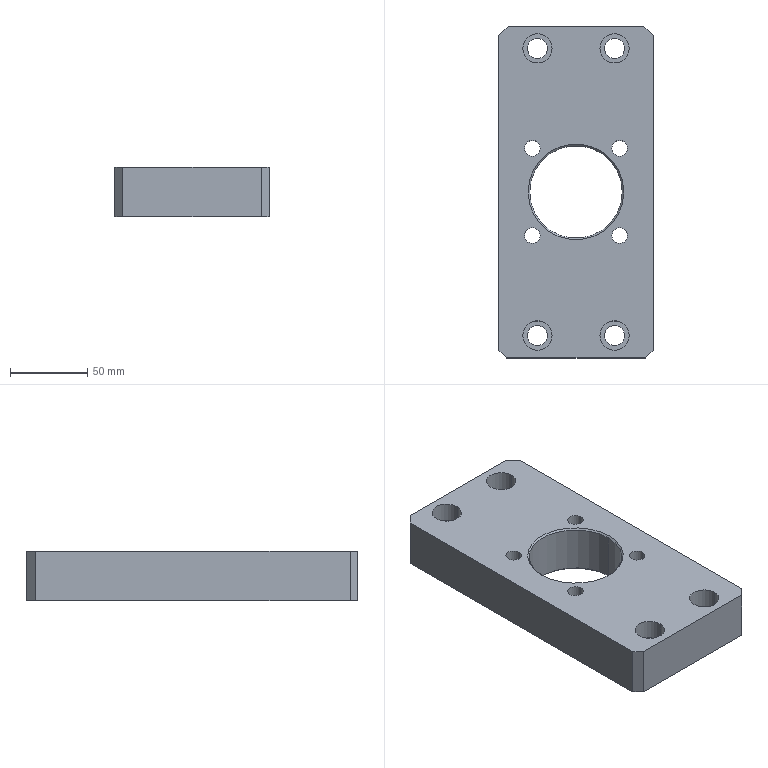Part | SolidWorks | features BaseBody 1 | 1 solid | 44 faces | box 100 x 215 x 32 mm | volume 560281 mm3 | cylinder 26 | plane 14 | cone 4 | commonest cylinder face diameters 10.106 x8 13 x8 19 x8 60 x2
STEP:
#1=CARTESIAN_POINT('',(146.031,36.728,1.));
#2=VERTEX_POINT('',#1);
#3=CARTESIAN_POINT('',(86.031,36.728,1.));
#4=VERTEX_POINT('',#3);
#5=CARTESIAN_POINT('',(116.031,36.728,1.));
#6=DIRECTION('',(0.,0.,-1.));
#7=DIRECTION('',(-1.,0.,0.));
#8=AXIS2_PLACEMENT_3D('',#5,#6,#7);
#9=CIRCLE('',#8,30.);
#10=EDGE_CURVE('',#2,#4,#9,.T.);
#11=ORIENTED_EDGE('',*,*,#10,.F.);
#12=CARTESIAN_POINT('',(147.031,36.728,0.));
#13=VERTEX_POINT('',#12);
#14=CARTESIAN_POINT('',(147.031,36.728,0.));
#15=DIRECTION('',(0.7071,0.,-0.7071));
#16=VECTOR('',#15,1000.);
#17=LINE('',#14,#16);
#18=EDGE_CURVE('',#2,#13,#17,.T.);
#19=ORIENTED_EDGE('',*,*,#18,.T.);
#20=CARTESIAN_POINT('',(85.031,36.728,0.));
#21=VERTEX_POINT('',#20);
#22=CARTESIAN_POINT('',(116.031,36.728,0.));
#23=DIRECTION('',(0.,0.,-1.));
#24=DIRECTION('',(-1.,0.,0.));
#25=AXIS2_PLACEMENT_3D('',#22,#23,#24);
#26=CIRCLE('',#25,31.);
#27=EDGE_CURVE('',#13,#21,#26,.T.);
#28=ORIENTED_EDGE('',*,*,#27,.T.);
#29=CARTESIAN_POINT('',(85.031,36.728,0.));
#30=DIRECTION('',(-0.7071,0.,-0.7071));
#31=VECTOR('',#30,1000.);
#32=LINE('',#29,#31);
#33=EDGE_CURVE('',#4,#21,#32,.T.);
#34=ORIENTED_EDGE('',*,*,#33,.F.);
#35=EDGE_LOOP('',(#11,#19,#28,#34));
#36=FACE_OUTER_BOUND('',#35,.T.);
#37=CARTESIAN_POINT('',(116.031,36.728,0.));
#38=DIRECTION('',(0.,0.,-1.));
#39=DIRECTION('',(-1.,0.,0.));
#40=AXIS2_PLACEMENT_3D('',#37,#38,#39);
#41=CONICAL_SURFACE('',#40,31.,0.7854);
#42=ADVANCED_FACE('',(#36),#41,.F.);
#43=CARTESIAN_POINT('',(92.799,8.444,0.));
#44=VERTEX_POINT('',#43);
#45=CARTESIAN_POINT('',(82.693,8.444,0.));
#46=VERTEX_POINT('',#45);
#47=CARTESIAN_POINT('',(87.746,8.444,0.));
#48=DIRECTION('',(0.,0.,-1.));
#49=DIRECTION('',(1.,0.,0.));
#50=AXIS2_PLACEMENT_3D('',#47,#48,#49);
#51=CIRCLE('',#50,5.053);
#52=EDGE_CURVE('',#44,#46,#51,.T.);
#53=ORIENTED_EDGE('',*,*,#52,.T.);
#54=CARTESIAN_POINT('',(82.693,8.444,32.));
#55=VERTEX_POINT('',#54);
#56=CARTESIAN_POINT('',(82.693,8.444,-207.268));
#57=DIRECTION('',(0.,0.,1.));
#58=VECTOR('',#57,1000.);
#59=LINE('',#56,#58);
#60=EDGE_CURVE('',#46,#55,#59,.T.);
#61=ORIENTED_EDGE('',*,*,#60,.T.);
#62=CARTESIAN_POINT('',(92.799,8.444,32.));
#63=VERTEX_POINT('',#62);
#64=CARTESIAN_POINT('',(87.746,8.444,32.));
#65=DIRECTION('',(0.,0.,-1.));
#66=DIRECTION('',(1.,0.,0.));
#67=AXIS2_PLACEMENT_3D('',#64,#65,#66);
#68=CIRCLE('',#67,5.053);
#69=EDGE_CURVE('',#63,#55,#68,.T.);
#70=ORIENTED_EDGE('',*,*,#69,.F.);
#71=CARTESIAN_POINT('',(92.799,8.444,-207.268));
#72=DIRECTION('',(0.,0.,1.));
#73=VECTOR('',#72,1000.);
#74=LINE('',#71,#73);
#75=EDGE_CURVE('',#44,#63,#74,.T.);
#76=ORIENTED_EDGE('',*,*,#75,.F.);
#77=EDGE_LOOP('',(#53,#61,#70,#76));
#78=FACE_OUTER_BOUND('',#77,.T.);
#79=CARTESIAN_POINT('',(87.746,8.444,-207.268));
#80=DIRECTION('',(0.,0.,1.));
#81=DIRECTION('',(1.,0.,0.));
#82=AXIS2_PLACEMENT_3D('',#79,#80,#81);
#83=CYLINDRICAL_SURFACE('',#82,5.053);
#84=ADVANCED_FACE('',(#78),#83,.F.);
#85=CARTESIAN_POINT('',(149.368,8.444,0.));
#86=VERTEX_POINT('',#85);
#87=CARTESIAN_POINT('',(139.262,8.444,0.));
#88=VERTEX_POINT('',#87);
#89=CARTESIAN_POINT('',(144.315,8.444,0.));
#90=DIRECTION('',(0.,0.,-1.));
#91=DIRECTION('',(1.,0.,0.));
#92=AXIS2_PLACEMENT_3D('',#89,#90,#91);
#93=CIRCLE('',#92,5.053);
#94=EDGE_CURVE('',#86,#88,#93,.T.);
#95=ORIENTED_EDGE('',*,*,#94,.T.);
#96=CARTESIAN_POINT('',(139.262,8.444,32.));
#97=VERTEX_POINT('',#96);
#98=CARTESIAN_POINT('',(139.262,8.444,-207.268));
#99=DIRECTION('',(0.,0.,1.));
#100=VECTOR('',#99,1000.);
#101=LINE('',#98,#100);
#102=EDGE_CURVE('',#88,#97,#101,.T.);
#103=ORIENTED_EDGE('',*,*,#102,.T.);
#104=CARTESIAN_POINT('',(149.368,8.444,32.));
#105=VERTEX_POINT('',#104);
#106=CARTESIAN_POINT('',(144.315,8.444,32.));
#107=DIRECTION('',(0.,0.,-1.));
#108=DIRECTION('',(1.,0.,0.));
#109=AXIS2_PLACEMENT_3D('',#106,#107,#108);
#110=CIRCLE('',#109,5.053);
#111=EDGE_CURVE('',#105,#97,#110,.T.);
#112=ORIENTED_EDGE('',*,*,#111,.F.);
#113=CARTESIAN_POINT('',(149.368,8.444,-207.268));
#114=DIRECTION('',(0.,0.,1.));
#115=VECTOR('',#114,1000.);
#116=LINE('',#113,#115);
#117=EDGE_CURVE('',#86,#105,#116,.T.);
#118=ORIENTED_EDGE('',*,*,#117,.F.);
#119=EDGE_LOOP('',(#95,#103,#112,#118));
#120=FACE_OUTER_BOUND('',#119,.T.);
#121=CARTESIAN_POINT('',(144.315,8.444,-207.268));
#122=DIRECTION('',(0.,0.,1.));
#123=DIRECTION('',(1.,0.,0.));
#124=AXIS2_PLACEMENT_3D('',#121,#122,#123);
#125=CYLINDRICAL_SURFACE('',#124,5.053);
#126=ADVANCED_FACE('',(#120),#125,.F.);
#127=CARTESIAN_POINT('',(149.368,65.013,0.));
#128=VERTEX_POINT('',#127);
#129=CARTESIAN_POINT('',(139.262,65.013,0.));
#130=VERTEX_POINT('',#129);
#131=CARTESIAN_POINT('',(144.315,65.013,0.));
#132=DIRECTION('',(0.,0.,-1.));
#133=DIRECTION('',(1.,0.,0.));
#134=AXIS2_PLACEMENT_3D('',#131,#132,#133);
#135=CIRCLE('',#134,5.053);
#136=EDGE_CURVE('',#128,#130,#135,.T.);
#137=ORIENTED_EDGE('',*,*,#136,.T.);
#138=CARTESIAN_POINT('',(139.262,65.013,32.));
#139=VERTEX_POINT('',#138);
#140=CARTESIAN_POINT('',(139.262,65.013,-207.268));
#141=DIRECTION('',(0.,0.,1.));
#142=VECTOR('',#141,1000.);
#143=LINE('',#140,#142);
#144=EDGE_CURVE('',#130,#139,#143,.T.);
#145=ORIENTED_EDGE('',*,*,#144,.T.);
#146=CARTESIAN_POINT('',(149.368,65.013,32.));
#147=VERTEX_POINT('',#146);
#148=CARTESIAN_POINT('',(144.315,65.013,32.));
#149=DIRECTION('',(0.,0.,-1.));
#150=DIRECTION('',(1.,0.,0.));
#151=AXIS2_PLACEMENT_3D('',#148,#149,#150);
#152=CIRCLE('',#151,5.053);
#153=EDGE_CURVE('',#147,#139,#152,.T.);
#154=ORIENTED_EDGE('',*,*,#153,.F.);
#155=CARTESIAN_POINT('',(149.368,65.013,-207.268));
#156=DIRECTION('',(0.,0.,1.));
#157=VECTOR('',#156,1000.);
#158=LINE('',#155,#157);
#159=EDGE_CURVE('',#128,#147,#158,.T.);
#160=ORIENTED_EDGE('',*,*,#159,.F.);
#161=EDGE_LOOP('',(#137,#145,#154,#160));
#162=FACE_OUTER_BOUND('',#161,.T.);
#163=CARTESIAN_POINT('',(144.315,65.013,-207.268));
#164=DIRECTION('',(0.,0.,1.));
#165=DIRECTION('',(1.,0.,0.));
#166=AXIS2_PLACEMENT_3D('',#163,#164,#165);
#167=CYLINDRICAL_SURFACE('',#166,5.053);
#168=ADVANCED_FACE('',(#162),#167,.F.);
#169=CARTESIAN_POINT('',(92.799,65.013,0.));
#170=VERTEX_POINT('',#169);
#171=CARTESIAN_POINT('',(82.693,65.013,0.));
#172=VERTEX_POINT('',#171);
#173=CARTESIAN_POINT('',(87.746,65.013,0.));
#174=DIRECTION('',(0.,0.,-1.));
#175=DIRECTION('',(1.,0.,0.));
#176=AXIS2_PLACEMENT_3D('',#173,#174,#175);
#177=CIRCLE('',#176,5.053);
#178=EDGE_CURVE('',#170,#172,#177,.T.);
#179=ORIENTED_EDGE('',*,*,#178,.T.);
#180=CARTESIAN_POINT('',(82.693,65.013,32.));
#181=VERTEX_POINT('',#180);
#182=CARTESIAN_POINT('',(82.693,65.013,-207.268));
#183=DIRECTION('',(0.,0.,1.));
#184=VECTOR('',#183,1000.);
#185=LINE('',#182,#184);
#186=EDGE_CURVE('',#172,#181,#185,.T.);
#187=ORIENTED_EDGE('',*,*,#186,.T.);
#188=CARTESIAN_POINT('',(92.799,65.013,32.));
#189=VERTEX_POINT('',#188);
#190=CARTESIAN_POINT('',(87.746,65.013,32.));
#191=DIRECTION('',(0.,0.,-1.));
#192=DIRECTION('',(1.,0.,0.));
#193=AXIS2_PLACEMENT_3D('',#190,#191,#192);
#194=CIRCLE('',#193,5.053);
#195=EDGE_CURVE('',#189,#181,#194,.T.);
#196=ORIENTED_EDGE('',*,*,#195,.F.);
#197=CARTESIAN_POINT('',(92.799,65.013,-207.268));
#198=DIRECTION('',(0.,0.,1.));
#199=VECTOR('',#198,1000.);
#200=LINE('',#197,#199);
#201=EDGE_CURVE('',#170,#189,#200,.T.);
#202=ORIENTED_EDGE('',*,*,#201,.F.);
#203=EDGE_LOOP('',(#179,#187,#196,#202));
#204=FACE_OUTER_BOUND('',#203,.T.);
#205=CARTESIAN_POINT('',(87.746,65.013,-207.268));
#206=DIRECTION('',(0.,0.,1.));
#207=DIRECTION('',(1.,0.,0.));
#208=AXIS2_PLACEMENT_3D('',#205,#206,#207);
#209=CYLINDRICAL_SURFACE('',#208,5.053);
#210=ADVANCED_FACE('',(#204),#209,.F.);
#211=CARTESIAN_POINT('',(97.531,-56.272,0.));
#212=VERTEX_POINT('',#211);
#213=CARTESIAN_POINT('',(84.531,-56.272,0.));
#214=VERTEX_POINT('',#213);
#215=CARTESIAN_POINT('',(91.031,-56.272,0.));
#216=DIRECTION('',(0.,0.,-1.));
#217=DIRECTION('',(1.,0.,0.));
#218=AXIS2_PLACEMENT_3D('',#215,#216,#217);
#219=CIRCLE('',#218,6.5);
#220=EDGE_CURVE('',#212,#214,#219,.T.);
#221=ORIENTED_EDGE('',*,*,#220,.T.);
#222=CARTESIAN_POINT('',(84.531,-56.272,19.));
#223=VERTEX_POINT('',#222);
#224=CARTESIAN_POINT('',(84.531,-56.272,-207.268));
#225=DIRECTION('',(0.,0.,1.));
#226=VECTOR('',#225,1000.);
#227=LINE('',#224,#226);
#228=EDGE_CURVE('',#214,#223,#227,.T.);
#229=ORIENTED_EDGE('',*,*,#228,.T.);
#230=CARTESIAN_POINT('',(97.531,-56.272,19.));
#231=VERTEX_POINT('',#230);
#232=CARTESIAN_POINT('',(91.031,-56.272,19.));
#233=DIRECTION('',(0.,0.,-1.));
#234=DIRECTION('',(1.,0.,0.));
#235=AXIS2_PLACEMENT_3D('',#232,#233,#234);
#236=CIRCLE('',#235,6.5);
#237=EDGE_CURVE('',#231,#223,#236,.T.);
#238=ORIENTED_EDGE('',*,*,#237,.F.);
#239=CARTESIAN_POINT('',(97.531,-56.272,-207.268));
#240=DIRECTION('',(0.,0.,1.));
#241=VECTOR('',#240,1000.);
#242=LINE('',#239,#241);
#243=EDGE_CURVE('',#212,#231,#242,.T.);
#244=ORIENTED_EDGE('',*,*,#243,.F.);
#245=EDGE_LOOP('',(#221,#229,#238,#244));
#246=FACE_OUTER_BOUND('',#245,.T.);
#247=CARTESIAN_POINT('',(91.031,-56.272,-207.268));
#248=DIRECTION('',(0.,0.,1.));
#249=DIRECTION('',(1.,0.,0.));
#250=AXIS2_PLACEMENT_3D('',#247,#248,#249);
#251=CYLINDRICAL_SURFACE('',#250,6.5);
#252=ADVANCED_FACE('',(#246),#251,.F.);
#253=CARTESIAN_POINT('',(147.531,-56.272,0.));
#254=VERTEX_POINT('',#253);
#255=CARTESIAN_POINT('',(134.531,-56.272,0.));
#256=VERTEX_POINT('',#255);
#257=CARTESIAN_POINT('',(141.031,-56.272,0.));
#258=DIRECTION('',(0.,0.,-1.));
#259=DIRECTION('',(1.,0.,0.));
#260=AXIS2_PLACEMENT_3D('',#257,#258,#259);
#261=CIRCLE('',#260,6.5);
#262=EDGE_CURVE('',#254,#256,#261,.T.);
#263=ORIENTED_EDGE('',*,*,#262,.T.);
#264=CARTESIAN_POINT('',(134.531,-56.272,19.));
#265=VERTEX_POINT('',#264);
#266=CARTESIAN_POINT('',(134.531,-56.272,-207.268));
#267=DIRECTION('',(0.,0.,1.));
#268=VECTOR('',#267,1000.);
#269=LINE('',#266,#268);
#270=EDGE_CURVE('',#256,#265,#269,.T.);
#271=ORIENTED_EDGE('',*,*,#270,.T.);
#272=CARTESIAN_POINT('',(147.531,-56.272,19.));
#273=VERTEX_POINT('',#272);
#274=CARTESIAN_POINT('',(141.031,-56.272,19.));
#275=DIRECTION('',(0.,0.,-1.));
#276=DIRECTION('',(1.,0.,0.));
#277=AXIS2_PLACEMENT_3D('',#274,#275,#276);
#278=CIRCLE('',#277,6.5);
#279=EDGE_CURVE('',#273,#265,#278,.T.);
#280=ORIENTED_EDGE('',*,*,#279,.F.);
#281=CARTESIAN_POINT('',(147.531,-56.272,-207.268));
#282=DIRECTION('',(0.,0.,1.));
#283=VECTOR('',#282,1000.);
#284=LINE('',#281,#283);
#285=EDGE_CURVE('',#254,#273,#284,.T.);
#286=ORIENTED_EDGE('',*,*,#285,.F.);
#287=EDGE_LOOP('',(#263,#271,#280,#286));
#288=FACE_OUTER_BOUND('',#287,.T.);
#289=CARTESIAN_POINT('',(141.031,-56.272,-207.268));
#290=DIRECTION('',(0.,0.,1.));
#291=DIRECTION('',(1.,0.,0.));
#292=AXIS2_PLACEMENT_3D('',#289,#290,#291);
#293=CYLINDRICAL_SURFACE('',#292,6.5);
#294=ADVANCED_FACE('',(#288),#293,.F.);
#295=CARTESIAN_POINT('',(147.531,129.728,0.));
#296=VERTEX_POINT('',#295);
#297=CARTESIAN_POINT('',(134.531,129.728,0.));
#298=VERTEX_POINT('',#297);
#299=CARTESIAN_POINT('',(141.031,129.728,0.));
#300=DIRECTION('',(0.,0.,-1.));
#301=DIRECTION('',(1.,0.,0.));
#302=AXIS2_PLACEMENT_3D('',#299,#300,#301);
#303=CIRCLE('',#302,6.5);
#304=EDGE_CURVE('',#296,#298,#303,.T.);
#305=ORIENTED_EDGE('',*,*,#304,.T.);
#306=CARTESIAN_POINT('',(134.531,129.728,19.));
#307=VERTEX_POINT('',#306);
#308=CARTESIAN_POINT('',(134.531,129.728,-207.268));
#309=DIRECTION('',(0.,0.,1.));
#310=VECTOR('',#309,1000.);
#311=LINE('',#308,#310);
#312=EDGE_CURVE('',#298,#307,#311,.T.);
#313=ORIENTED_EDGE('',*,*,#312,.T.);
#314=CARTESIAN_POINT('',(147.531,129.728,19.));
#315=VERTEX_POINT('',#314);
#316=CARTESIAN_POINT('',(141.031,129.728,19.));
#317=DIRECTION('',(0.,0.,-1.));
#318=DIRECTION('',(1.,0.,0.));
#319=AXIS2_PLACEMENT_3D('',#316,#317,#318);
#320=CIRCLE('',#319,6.5);
#321=EDGE_CURVE('',#315,#307,#320,.T.);
#322=ORIENTED_EDGE('',*,*,#321,.F.);
#323=CARTESIAN_POINT('',(147.531,129.728,-207.268));
#324=DIRECTION('',(0.,0.,1.));
#325=VECTOR('',#324,1000.);
#326=LINE('',#323,#325);
#327=EDGE_CURVE('',#296,#315,#326,.T.);
#328=ORIENTED_EDGE('',*,*,#327,.F.);
#329=EDGE_LOOP('',(#305,#313,#322,#328));
#330=FACE_OUTER_BOUND('',#329,.T.);
#331=CARTESIAN_POINT('',(141.031,129.728,-207.268));
#332=DIRECTION('',(0.,0.,1.));
#333=DIRECTION('',(1.,0.,0.));
#334=AXIS2_PLACEMENT_3D('',#331,#332,#333);
#335=CYLINDRICAL_SURFACE('',#334,6.5);
#336=ADVANCED_FACE('',(#330),#335,.F.);
#337=CARTESIAN_POINT('',(97.531,129.728,0.));
#338=VERTEX_POINT('',#337);
#339=CARTESIAN_POINT('',(84.531,129.728,0.));
#340=VERTEX_POINT('',#339);
#341=CARTESIAN_POINT('',(91.031,129.728,0.));
#342=DIRECTION('',(0.,0.,-1.));
#343=DIRECTION('',(1.,0.,0.));
#344=AXIS2_PLACEMENT_3D('',#341,#342,#343);
#345=CIRCLE('',#344,6.5);
#346=EDGE_CURVE('',#338,#340,#345,.T.);
#347=ORIENTED_EDGE('',*,*,#346,.T.);
#348=CARTESIAN_POINT('',(84.531,129.728,19.));
#349=VERTEX_POINT('',#348);
#350=CARTESIAN_POINT('',(84.531,129.728,-207.268));
#351=DIRECTION('',(0.,0.,1.));
#352=VECTOR('',#351,1000.);
#353=LINE('',#350,#352);
#354=EDGE_CURVE('',#340,#349,#353,.T.);
#355=ORIENTED_EDGE('',*,*,#354,.T.);
#356=CARTESIAN_POINT('',(97.531,129.728,19.));
#357=VERTEX_POINT('',#356);
#358=CARTESIAN_POINT('',(91.031,129.728,19.));
#359=DIRECTION('',(0.,0.,-1.));
#360=DIRECTION('',(1.,0.,0.));
#361=AXIS2_PLACEMENT_3D('',#358,#359,#360);
#362=CIRCLE('',#361,6.5);
#363=EDGE_CURVE('',#357,#349,#362,.T.);
#364=ORIENTED_EDGE('',*,*,#363,.F.);
#365=CARTESIAN_POINT('',(97.531,129.728,-207.268));
#366=DIRECTION('',(0.,0.,1.));
#367=VECTOR('',#366,1000.);
#368=LINE('',#365,#367);
#369=EDGE_CURVE('',#338,#357,#368,.T.);
#370=ORIENTED_EDGE('',*,*,#369,.F.);
#371=EDGE_LOOP('',(#347,#355,#364,#370));
#372=FACE_OUTER_BOUND('',#371,.T.);
#373=CARTESIAN_POINT('',(91.031,129.728,-207.268));
#374=DIRECTION('',(0.,0.,1.));
#375=DIRECTION('',(1.,0.,0.));
#376=AXIS2_PLACEMENT_3D('',#373,#374,#375);
#377=CYLINDRICAL_SURFACE('',#376,6.5);
#378=ADVANCED_FACE('',(#372),#377,.F.);
#379=ORIENTED_EDGE('',*,*,#10,.T.);
#380=CARTESIAN_POINT('',(86.031,36.728,31.));
#381=VERTEX_POINT('',#380);
#382=CARTESIAN_POINT('',(86.031,36.728,0.));
#383=DIRECTION('',(0.,0.,1.));
#384=VECTOR('',#383,1000.);
#385=LINE('',#382,#384);
#386=EDGE_CURVE('',#4,#381,#385,.T.);
#387=ORIENTED_EDGE('',*,*,#386,.T.);
#388=CARTESIAN_POINT('',(146.031,36.728,31.));
#389=VERTEX_POINT('',#388);
#390=CARTESIAN_POINT('',(116.031,36.728,31.));
#391=DIRECTION('',(0.,0.,-1.));
#392=DIRECTION('',(1.,0.,0.));
#393=AXIS2_PLACEMENT_3D('',#390,#391,#392);
#394=CIRCLE('',#393,30.);
#395=EDGE_CURVE('',#389,#381,#394,.T.);
#396=ORIENTED_EDGE('',*,*,#395,.F.);
#397=CARTESIAN_POINT('',(146.031,36.728,0.));
#398=DIRECTION('',(0.,0.,1.));
#399=VECTOR('',#398,1000.);
#400=LINE('',#397,#399);
#401=EDGE_CURVE('',#2,#389,#400,.T.);
#402=ORIENTED_EDGE('',*,*,#401,.F.);
#403=EDGE_LOOP('',(#379,#387,#396,#402));
#404=FACE_OUTER_BOUND('',#403,.T.);
#405=CARTESIAN_POINT('',(116.031,36.728,0.));
#406=DIRECTION('',(0.,0.,1.));
#407=DIRECTION('',(1.,0.,0.));
#408=AXIS2_PLACEMENT_3D('',#405,#406,#407);
#409=CYLINDRICAL_SURFACE('',#408,30.);
#410=ADVANCED_FACE('',(#404),#409,.F.);
#411=ORIENTED_EDGE('',*,*,#395,.T.);
#412=CARTESIAN_POINT('',(85.031,36.728,32.));
#413=VERTEX_POINT('',#412);
#414=CARTESIAN_POINT('',(85.031,36.728,32.));
#415=DIRECTION('',(-0.7071,0.,0.7071));
#416=VECTOR('',#415,1000.);
#417=LINE('',#414,#416);
#418=EDGE_CURVE('',#381,#413,#417,.T.);
#419=ORIENTED_EDGE('',*,*,#418,.T.);
#420=CARTESIAN_POINT('',(147.031,36.728,32.));
#421=VERTEX_POINT('',#420);
#422=CARTESIAN_POINT('',(116.031,36.728,32.));
#423=DIRECTION('',(0.,0.,-1.));
#424=DIRECTION('',(1.,0.,0.));
#425=AXIS2_PLACEMENT_3D('',#422,#423,#424);
#426=CIRCLE('',#425,31.);
#427=EDGE_CURVE('',#421,#413,#426,.T.);
#428=ORIENTED_EDGE('',*,*,#427,.F.);
#429=CARTESIAN_POINT('',(147.031,36.728,32.));
#430=DIRECTION('',(0.7071,0.,0.7071));
#431=VECTOR('',#430,1000.);
#432=LINE('',#429,#431);
#433=EDGE_CURVE('',#389,#421,#432,.T.);
#434=ORIENTED_EDGE('',*,*,#433,.F.);
#435=EDGE_LOOP('',(#411,#419,#428,#434));
#436=FACE_OUTER_BOUND('',#435,.T.);
#437=CARTESIAN_POINT('',(116.031,36.728,32.));
#438=DIRECTION('',(0.,0.,1.));
#439=DIRECTION('',(1.,0.,0.));
#440=AXIS2_PLACEMENT_3D('',#437,#438,#439);
#441=CONICAL_SURFACE('',#440,31.,0.7854);
#442=ADVANCED_FACE('',(#436),#441,.F.);
#443=CARTESIAN_POINT('',(81.531,-56.272,19.));
#444=VERTEX_POINT('',#443);
#445=CARTESIAN_POINT('',(100.531,-56.272,19.));
#446=VERTEX_POINT('',#445);
#447=CARTESIAN_POINT('',(91.031,-56.272,19.));
#448=DIRECTION('',(0.,0.,1.));
#449=DIRECTION('',(1.,0.,0.));
#450=AXIS2_PLACEMENT_3D('',#447,#448,#449);
#451=CIRCLE('',#450,9.5);
#452=EDGE_CURVE('',#444,#446,#451,.T.);
#453=ORIENTED_EDGE('',*,*,#452,.F.);
#454=CARTESIAN_POINT('',(81.531,-56.272,32.));
#455=VERTEX_POINT('',#454);
#456=CARTESIAN_POINT('',(81.531,-56.272,25.5));
#457=DIRECTION('',(0.,0.,1.));
#458=VECTOR('',#457,1000.);
#459=LINE('',#456,#458);
#460=EDGE_CURVE('',#444,#455,#459,.T.);
#461=ORIENTED_EDGE('',*,*,#460,.T.);
#462=CARTESIAN_POINT('',(100.531,-56.272,32.));
#463=VERTEX_POINT('',#462);
#464=CARTESIAN_POINT('',(91.031,-56.272,32.));
#465=DIRECTION('',(0.,0.,-1.));
#466=DIRECTION('',(1.,0.,0.));
#467=AXIS2_PLACEMENT_3D('',#464,#465,#466);
#468=CIRCLE('',#467,9.5);
#469=EDGE_CURVE('',#463,#455,#468,.T.);
#470=ORIENTED_EDGE('',*,*,#469,.F.);
#471=CARTESIAN_POINT('',(100.531,-56.272,25.5));
#472=DIRECTION('',(0.,0.,1.));
#473=VECTOR('',#472,1000.);
#474=LINE('',#471,#473);
#475=EDGE_CURVE('',#446,#463,#474,.T.);
#476=ORIENTED_EDGE('',*,*,#475,.F.);
#477=EDGE_LOOP('',(#453,#461,#470,#476));
#478=FACE_OUTER_BOUND('',#477,.T.);
#479=CARTESIAN_POINT('',(91.031,-56.272,25.5));
#480=DIRECTION('',(0.,0.,1.));
#481=DIRECTION('',(1.,0.,0.));
#482=AXIS2_PLACEMENT_3D('',#479,#480,#481);
#483=CYLINDRICAL_SURFACE('',#482,9.5);
#484=ADVANCED_FACE('',(#478),#483,.F.);
#485=CARTESIAN_POINT('',(131.531,-56.272,19.));
#486=VERTEX_POINT('',#485);
#487=CARTESIAN_POINT('',(150.531,-56.272,19.));
#488=VERTEX_POINT('',#487);
#489=CARTESIAN_POINT('',(141.031,-56.272,19.));
#490=DIRECTION('',(0.,0.,1.));
#491=DIRECTION('',(1.,0.,0.));
#492=AXIS2_PLACEMENT_3D('',#489,#490,#491);
#493=CIRCLE('',#492,9.5);
#494=EDGE_CURVE('',#486,#488,#493,.T.);
#495=ORIENTED_EDGE('',*,*,#494,.F.);
#496=CARTESIAN_POINT('',(131.531,-56.272,32.));
#497=VERTEX_POINT('',#496);
#498=CARTESIAN_POINT('',(131.531,-56.272,25.5));
#499=DIRECTION('',(0.,0.,1.));
#500=VECTOR('',#499,1000.);
#501=LINE('',#498,#500);
#502=EDGE_CURVE('',#486,#497,#501,.T.);
#503=ORIENTED_EDGE('',*,*,#502,.T.);
#504=CARTESIAN_POINT('',(150.531,-56.272,32.));
#505=VERTEX_POINT('',#504);
#506=CARTESIAN_POINT('',(141.031,-56.272,32.));
#507=DIRECTION('',(0.,0.,-1.));
#508=DIRECTION('',(1.,0.,0.));
#509=AXIS2_PLACEMENT_3D('',#506,#507,#508);
#510=CIRCLE('',#509,9.5);
#511=EDGE_CURVE('',#505,#497,#510,.T.);
#512=ORIENTED_EDGE('',*,*,#511,.F.);
#513=CARTESIAN_POINT('',(150.531,-56.272,25.5));
#514=DIRECTION('',(0.,0.,1.));
#515=VECTOR('',#514,1000.);
#516=LINE('',#513,#515);
#517=EDGE_CURVE('',#488,#505,#516,.T.);
#518=ORIENTED_EDGE('',*,*,#517,.F.);
#519=EDGE_LOOP('',(#495,#503,#512,#518));
#520=FACE_OUTER_BOUND('',#519,.T.);
#521=CARTESIAN_POINT('',(141.031,-56.272,25.5));
#522=DIRECTION('',(0.,0.,1.));
#523=DIRECTION('',(1.,0.,0.));
#524=AXIS2_PLACEMENT_3D('',#521,#522,#523);
#525=CYLINDRICAL_SURFACE('',#524,9.5);
#526=ADVANCED_FACE('',(#520),#525,.F.);
#527=CARTESIAN_POINT('',(131.531,129.728,19.));
#528=VERTEX_POINT('',#527);
#529=CARTESIAN_POINT('',(150.531,129.728,19.));
#530=VERTEX_POINT('',#529);
#531=CARTESIAN_POINT('',(141.031,129.728,19.));
#532=DIRECTION('',(0.,0.,1.));
#533=DIRECTION('',(1.,0.,0.));
#534=AXIS2_PLACEMENT_3D('',#531,#532,#533);
#535=CIRCLE('',#534,9.5);
#536=EDGE_CURVE('',#528,#530,#535,.T.);
#537=ORIENTED_EDGE('',*,*,#536,.F.);
#538=CARTESIAN_POINT('',(131.531,129.728,32.));
#539=VERTEX_POINT('',#538);
#540=CARTESIAN_POINT('',(131.531,129.728,25.5));
#541=DIRECTION('',(0.,0.,1.));
#542=VECTOR('',#541,1000.);
#543=LINE('',#540,#542);
#544=EDGE_CURVE('',#528,#539,#543,.T.);
#545=ORIENTED_EDGE('',*,*,#544,.T.);
#546=CARTESIAN_POINT('',(150.531,129.728,32.));
#547=VERTEX_POINT('',#546);
#548=CARTESIAN_POINT('',(141.031,129.728,32.));
#549=DIRECTION('',(0.,0.,-1.));
#550=DIRECTION('',(1.,0.,0.));
#551=AXIS2_PLACEMENT_3D('',#548,#549,#550);
#552=CIRCLE('',#551,9.5);
#553=EDGE_CURVE('',#547,#539,#552,.T.);
#554=ORIENTED_EDGE('',*,*,#553,.F.);
#555=CARTESIAN_POINT('',(150.531,129.728,25.5));
#556=DIRECTION('',(0.,0.,1.));
#557=VECTOR('',#556,1000.);
#558=LINE('',#555,#557);
#559=EDGE_CURVE('',#530,#547,#558,.T.);
#560=ORIENTED_EDGE('',*,*,#559,.F.);
#561=EDGE_LOOP('',(#537,#545,#554,#560));
#562=FACE_OUTER_BOUND('',#561,.T.);
#563=CARTESIAN_POINT('',(141.031,129.728,25.5));
#564=DIRECTION('',(0.,0.,1.));
#565=DIRECTION('',(1.,0.,0.));
#566=AXIS2_PLACEMENT_3D('',#563,#564,#565);
#567=CYLINDRICAL_SURFACE('',#566,9.5);
#568=ADVANCED_FACE('',(#562),#567,.F.);
#569=CARTESIAN_POINT('',(81.531,129.728,19.));
#570=VERTEX_POINT('',#569);
#571=CARTESIAN_POINT('',(100.531,129.728,19.));
#572=VERTEX_POINT('',#571);
#573=CARTESIAN_POINT('',(91.031,129.728,19.));
#574=DIRECTION('',(0.,0.,1.));
#575=DIRECTION('',(1.,0.,0.));
#576=AXIS2_PLACEMENT_3D('',#573,#574,#575);
#577=CIRCLE('',#576,9.5);
#578=EDGE_CURVE('',#570,#572,#577,.T.);
#579=ORIENTED_EDGE('',*,*,#578,.F.);
#580=CARTESIAN_POINT('',(81.531,129.728,32.));
#581=VERTEX_POINT('',#580);
#582=CARTESIAN_POINT('',(81.531,129.728,25.5));
#583=DIRECTION('',(0.,0.,1.));
#584=VECTOR('',#583,1000.);
#585=LINE('',#582,#584);
#586=EDGE_CURVE('',#570,#581,#585,.T.);
#587=ORIENTED_EDGE('',*,*,#586,.T.);
#588=CARTESIAN_POINT('',(100.531,129.728,32.));
#589=VERTEX_POINT('',#588);
#590=CARTESIAN_POINT('',(91.031,129.728,32.));
#591=DIRECTION('',(0.,0.,-1.));
#592=DIRECTION('',(1.,0.,0.));
#593=AXIS2_PLACEMENT_3D('',#590,#591,#592);
#594=CIRCLE('',#593,9.5);
#595=EDGE_CURVE('',#589,#581,#594,.T.);
#596=ORIENTED_EDGE('',*,*,#595,.F.);
#597=CARTESIAN_POINT('',(100.531,129.728,25.5));
#598=DIRECTION('',(0.,0.,1.));
#599=VECTOR('',#598,1000.);
#600=LINE('',#597,#599);
#601=EDGE_CURVE('',#572,#589,#600,.T.);
#602=ORIENTED_EDGE('',*,*,#601,.F.);
#603=EDGE_LOOP('',(#579,#587,#596,#602));
#604=FACE_OUTER_BOUND('',#603,.T.);
#605=CARTESIAN_POINT('',(91.031,129.728,25.5));
#606=DIRECTION('',(0.,0.,1.));
#607=DIRECTION('',(1.,0.,0.));
#608=AXIS2_PLACEMENT_3D('',#605,#606,#607);
#609=CYLINDRICAL_SURFACE('',#608,9.5);
#610=ADVANCED_FACE('',(#604),#609,.F.);
#611=CARTESIAN_POINT('',(116.031,36.728,0.));
#612=DIRECTION('',(0.,0.,-1.));
#613=DIRECTION('',(-1.,0.,0.));
#614=AXIS2_PLACEMENT_3D('',#611,#612,#613);
#615=CIRCLE('',#614,31.);
#616=EDGE_CURVE('',#21,#13,#615,.T.);
#617=ORIENTED_EDGE('',*,*,#616,.F.);
#618=ORIENTED_EDGE('',*,*,#27,.F.);
#619=EDGE_LOOP('',(#617,#618));
#620=FACE_BOUND('',#619,.T.);
#621=ORIENTED_EDGE('',*,*,#52,.F.);
#622=CARTESIAN_POINT('',(87.746,8.444,0.));
#623=DIRECTION('',(0.,0.,-1.));
#624=DIRECTION('',(1.,0.,0.));
#625=AXIS2_PLACEMENT_3D('',#622,#623,#624);
#626=CIRCLE('',#625,5.053);
#627=EDGE_CURVE('',#46,#44,#626,.T.);
#628=ORIENTED_EDGE('',*,*,#627,.F.);
#629=EDGE_LOOP('',(#621,#628));
#630=FACE_BOUND('',#629,.T.);
#631=ORIENTED_EDGE('',*,*,#94,.F.);
#632=CARTESIAN_POINT('',(144.315,8.444,0.));
#633=DIRECTION('',(0.,0.,-1.));
#634=DIRECTION('',(1.,0.,0.));
#635=AXIS2_PLACEMENT_3D('',#632,#633,#634);
#636=CIRCLE('',#635,5.053);
#637=EDGE_CURVE('',#88,#86,#636,.T.);
#638=ORIENTED_EDGE('',*,*,#637,.F.);
#639=EDGE_LOOP('',(#631,#638));
#640=FACE_BOUND('',#639,.T.);
#641=ORIENTED_EDGE('',*,*,#136,.F.);
#642=CARTESIAN_POINT('',(144.315,65.013,0.));
#643=DIRECTION('',(0.,0.,-1.));
#644=DIRECTION('',(1.,0.,0.));
#645=AXIS2_PLACEMENT_3D('',#642,#643,#644);
#646=CIRCLE('',#645,5.053);
#647=EDGE_CURVE('',#130,#128,#646,.T.);
#648=ORIENTED_EDGE('',*,*,#647,.F.);
#649=EDGE_LOOP('',(#641,#648));
#650=FACE_BOUND('',#649,.T.);
#651=ORIENTED_EDGE('',*,*,#178,.F.);
#652=CARTESIAN_POINT('',(87.746,65.013,0.));
#653=DIRECTION('',(0.,0.,-1.));
#654=DIRECTION('',(1.,0.,0.));
#655=AXIS2_PLACEMENT_3D('',#652,#653,#654);
#656=CIRCLE('',#655,5.053);
#657=EDGE_CURVE('',#172,#170,#656,.T.);
#658=ORIENTED_EDGE('',*,*,#657,.F.);
#659=EDGE_LOOP('',(#651,#658));
#660=FACE_BOUND('',#659,.T.);
#661=ORIENTED_EDGE('',*,*,#220,.F.);
#662=CARTESIAN_POINT('',(91.031,-56.272,0.));
#663=DIRECTION('',(0.,0.,-1.));
#664=DIRECTION('',(1.,0.,0.));
#665=AXIS2_PLACEMENT_3D('',#662,#663,#664);
#666=CIRCLE('',#665,6.5);
#667=EDGE_CURVE('',#214,#212,#666,.T.);
#668=ORIENTED_EDGE('',*,*,#667,.F.);
#669=EDGE_LOOP('',(#661,#668));
#670=FACE_BOUND('',#669,.T.);
#671=ORIENTED_EDGE('',*,*,#262,.F.);
#672=CARTESIAN_POINT('',(141.031,-56.272,0.));
#673=DIRECTION('',(0.,0.,-1.));
#674=DIRECTION('',(1.,0.,0.));
#675=AXIS2_PLACEMENT_3D('',#672,#673,#674);
#676=CIRCLE('',#675,6.5);
#677=EDGE_CURVE('',#256,#254,#676,.T.);
#678=ORIENTED_EDGE('',*,*,#677,.F.);
#679=EDGE_LOOP('',(#671,#678));
#680=FACE_BOUND('',#679,.T.);
#681=ORIENTED_EDGE('',*,*,#304,.F.);
#682=CARTESIAN_POINT('',(141.031,129.728,0.));
#683=DIRECTION('',(0.,0.,-1.));
#684=DIRECTION('',(1.,0.,0.));
#685=AXIS2_PLACEMENT_3D('',#682,#683,#684);
#686=CIRCLE('',#685,6.5);
#687=EDGE_CURVE('',#298,#296,#686,.T.);
#688=ORIENTED_EDGE('',*,*,#687,.F.);
#689=EDGE_LOOP('',(#681,#688));
#690=FACE_BOUND('',#689,.T.);
#691=ORIENTED_EDGE('',*,*,#346,.F.);
#692=CARTESIAN_POINT('',(91.031,129.728,0.));
#693=DIRECTION('',(0.,0.,-1.));
#694=DIRECTION('',(1.,0.,0.));
#695=AXIS2_PLACEMENT_3D('',#692,#693,#694);
#696=CIRCLE('',#695,6.5);
#697=EDGE_CURVE('',#340,#338,#696,.T.);
#698=ORIENTED_EDGE('',*,*,#697,.F.);
#699=EDGE_LOOP('',(#691,#698));
#700=FACE_BOUND('',#699,.T.);
#701=CARTESIAN_POINT('',(72.031,144.228,0.));
#702=VERTEX_POINT('',#701);
#703=CARTESIAN_POINT('',(66.031,138.228,0.));
#704=VERTEX_POINT('',#703);
#705=CARTESIAN_POINT('',(72.031,144.228,0.));
#706=DIRECTION('',(-0.7071,-0.7071,0.));
#707=VECTOR('',#706,1000.);
#708=LINE('',#705,#707);
#709=EDGE_CURVE('',#702,#704,#708,.T.);
#710=ORIENTED_EDGE('',*,*,#709,.F.);
#711=CARTESIAN_POINT('',(160.031,144.228,0.));
#712=VERTEX_POINT('',#711);
#713=CARTESIAN_POINT('',(116.031,144.228,0.));
#714=DIRECTION('',(-1.,0.,0.));
#715=VECTOR('',#714,1000.);
#716=LINE('',#713,#715);
#717=EDGE_CURVE('',#712,#702,#716,.T.);
#718=ORIENTED_EDGE('',*,*,#717,.F.);
#719=CARTESIAN_POINT('',(166.031,138.228,0.));
#720=VERTEX_POINT('',#719);
#721=CARTESIAN_POINT('',(166.031,138.228,0.));
#722=DIRECTION('',(-0.7071,0.7071,0.));
#723=VECTOR('',#722,1000.);
#724=LINE('',#721,#723);
#725=EDGE_CURVE('',#720,#712,#724,.T.);
#726=ORIENTED_EDGE('',*,*,#725,.F.);
#727=CARTESIAN_POINT('',(166.031,-65.772,0.));
#728=VERTEX_POINT('',#727);
#729=CARTESIAN_POINT('',(166.031,36.517,0.));
#730=DIRECTION('',(0.,1.,0.));
#731=VECTOR('',#730,1000.);
#732=LINE('',#729,#731);
#733=EDGE_CURVE('',#728,#720,#732,.T.);
#734=ORIENTED_EDGE('',*,*,#733,.F.);
#735=CARTESIAN_POINT('',(161.031,-70.772,0.));
#736=VERTEX_POINT('',#735);
#737=CARTESIAN_POINT('',(161.031,-70.772,0.));
#738=DIRECTION('',(0.7071,0.7071,0.));
#739=VECTOR('',#738,1000.);
#740=LINE('',#737,#739);
#741=EDGE_CURVE('',#736,#728,#740,.T.);
#742=ORIENTED_EDGE('',*,*,#741,.F.);
#743=CARTESIAN_POINT('',(71.031,-70.772,0.));
#744=VERTEX_POINT('',#743);
#745=CARTESIAN_POINT('',(116.031,-70.772,0.));
#746=DIRECTION('',(1.,0.,0.));
#747=VECTOR('',#746,1000.);
#748=LINE('',#745,#747);
#749=EDGE_CURVE('',#744,#736,#748,.T.);
#750=ORIENTED_EDGE('',*,*,#749,.F.);
#751=CARTESIAN_POINT('',(66.031,-65.772,0.));
#752=VERTEX_POINT('',#751);
#753=CARTESIAN_POINT('',(66.031,-65.772,0.));
#754=DIRECTION('',(0.7071,-0.7071,0.));
#755=VECTOR('',#754,1000.);
#756=LINE('',#753,#755);
#757=EDGE_CURVE('',#752,#744,#756,.T.);
#758=ORIENTED_EDGE('',*,*,#757,.F.);
#759=CARTESIAN_POINT('',(66.031,36.517,0.));
#760=DIRECTION('',(0.,-1.,0.));
#761=VECTOR('',#760,1000.);
#762=LINE('',#759,#761);
#763=EDGE_CURVE('',#704,#752,#762,.T.);
#764=ORIENTED_EDGE('',*,*,#763,.F.);
#765=EDGE_LOOP('',(#710,#718,#726,#734,#742,#750,#758,#764));
#766=FACE_OUTER_BOUND('',#765,.T.);
#767=CARTESIAN_POINT('',(116.031,36.517,0.));
#768=DIRECTION('',(0.,0.,1.));
#769=DIRECTION('',(1.,0.,0.));
#770=AXIS2_PLACEMENT_3D('',#767,#768,#769);
#771=PLANE('',#770);
#772=ADVANCED_FACE('',(#620,#630,#640,#650,#660,#670,#680,#690,#700,#766),#771,.F.);
#773=ORIENTED_EDGE('',*,*,#18,.F.);
#774=CARTESIAN_POINT('',(116.031,36.728,1.));
#775=DIRECTION('',(0.,0.,-1.));
#776=DIRECTION('',(-1.,0.,0.));
#777=AXIS2_PLACEMENT_3D('',#774,#775,#776);
#778=CIRCLE('',#777,30.);
#779=EDGE_CURVE('',#4,#2,#778,.T.);
#780=ORIENTED_EDGE('',*,*,#779,.F.);
#781=ORIENTED_EDGE('',*,*,#33,.T.);
#782=ORIENTED_EDGE('',*,*,#616,.T.);
#783=EDGE_LOOP('',(#773,#780,#781,#782));
#784=FACE_OUTER_BOUND('',#783,.T.);
#785=CARTESIAN_POINT('',(116.031,36.728,0.));
#786=DIRECTION('',(0.,0.,-1.));
#787=DIRECTION('',(-1.,0.,0.));
#788=AXIS2_PLACEMENT_3D('',#785,#786,#787);
#789=CONICAL_SURFACE('',#788,31.,0.7854);
#790=ADVANCED_FACE('',(#784),#789,.F.);
#791=ORIENTED_EDGE('',*,*,#60,.F.);
#792=ORIENTED_EDGE('',*,*,#627,.T.);
#793=ORIENTED_EDGE('',*,*,#75,.T.);
#794=CARTESIAN_POINT('',(87.746,8.444,32.));
#795=DIRECTION('',(0.,0.,-1.));
#796=DIRECTION('',(1.,0.,0.));
#797=AXIS2_PLACEMENT_3D('',#794,#795,#796);
#798=CIRCLE('',#797,5.053);
#799=EDGE_CURVE('',#55,#63,#798,.T.);
#800=ORIENTED_EDGE('',*,*,#799,.F.);
#801=EDGE_LOOP('',(#791,#792,#793,#800));
#802=FACE_OUTER_BOUND('',#801,.T.);
#803=CARTESIAN_POINT('',(87.746,8.444,-207.268));
#804=DIRECTION('',(0.,0.,1.));
#805=DIRECTION('',(1.,0.,0.));
#806=AXIS2_PLACEMENT_3D('',#803,#804,#805);
#807=CYLINDRICAL_SURFACE('',#806,5.053);
#808=ADVANCED_FACE('',(#802),#807,.F.);
#809=ORIENTED_EDGE('',*,*,#102,.F.);
#810=ORIENTED_EDGE('',*,*,#637,.T.);
#811=ORIENTED_EDGE('',*,*,#117,.T.);
#812=CARTESIAN_POINT('',(144.315,8.444,32.));
#813=DIRECTION('',(0.,0.,-1.));
#814=DIRECTION('',(1.,0.,0.));
#815=AXIS2_PLACEMENT_3D('',#812,#813,#814);
#816=CIRCLE('',#815,5.053);
#817=EDGE_CURVE('',#97,#105,#816,.T.);
#818=ORIENTED_EDGE('',*,*,#817,.F.);
#819=EDGE_LOOP('',(#809,#810,#811,#818));
#820=FACE_OUTER_BOUND('',#819,.T.);
#821=CARTESIAN_POINT('',(144.315,8.444,-207.268));
#822=DIRECTION('',(0.,0.,1.));
#823=DIRECTION('',(1.,0.,0.));
#824=AXIS2_PLACEMENT_3D('',#821,#822,#823);
#825=CYLINDRICAL_SURFACE('',#824,5.053);
#826=ADVANCED_FACE('',(#820),#825,.F.);
#827=ORIENTED_EDGE('',*,*,#144,.F.);
#828=ORIENTED_EDGE('',*,*,#647,.T.);
#829=ORIENTED_EDGE('',*,*,#159,.T.);
#830=CARTESIAN_POINT('',(144.315,65.013,32.));
#831=DIRECTION('',(0.,0.,-1.));
#832=DIRECTION('',(1.,0.,0.));
#833=AXIS2_PLACEMENT_3D('',#830,#831,#832);
#834=CIRCLE('',#833,5.053);
#835=EDGE_CURVE('',#139,#147,#834,.T.);
#836=ORIENTED_EDGE('',*,*,#835,.F.);
#837=EDGE_LOOP('',(#827,#828,#829,#836));
#838=FACE_OUTER_BOUND('',#837,.T.);
#839=CARTESIAN_POINT('',(144.315,65.013,-207.268));
#840=DIRECTION('',(0.,0.,1.));
#841=DIRECTION('',(1.,0.,0.));
#842=AXIS2_PLACEMENT_3D('',#839,#840,#841);
#843=CYLINDRICAL_SURFACE('',#842,5.053);
#844=ADVANCED_FACE('',(#838),#843,.F.);
#845=ORIENTED_EDGE('',*,*,#186,.F.);
#846=ORIENTED_EDGE('',*,*,#657,.T.);
#847=ORIENTED_EDGE('',*,*,#201,.T.);
#848=CARTESIAN_POINT('',(87.746,65.013,32.));
#849=DIRECTION('',(0.,0.,-1.));
#850=DIRECTION('',(1.,0.,0.));
#851=AXIS2_PLACEMENT_3D('',#848,#849,#850);
#852=CIRCLE('',#851,5.053);
#853=EDGE_CURVE('',#181,#189,#852,.T.);
#854=ORIENTED_EDGE('',*,*,#853,.F.);
#855=EDGE_LOOP('',(#845,#846,#847,#854));
#856=FACE_OUTER_BOUND('',#855,.T.);
#857=CARTESIAN_POINT('',(87.746,65.013,-207.268));
#858=DIRECTION('',(0.,0.,1.));
#859=DIRECTION('',(1.,0.,0.));
#860=AXIS2_PLACEMENT_3D('',#857,#858,#859);
#861=CYLINDRICAL_SURFACE('',#860,5.053);
#862=ADVANCED_FACE('',(#856),#861,.F.);
#863=ORIENTED_EDGE('',*,*,#228,.F.);
#864=ORIENTED_EDGE('',*,*,#667,.T.);
#865=ORIENTED_EDGE('',*,*,#243,.T.);
#866=CARTESIAN_POINT('',(91.031,-56.272,19.));
#867=DIRECTION('',(0.,0.,-1.));
#868=DIRECTION('',(1.,0.,0.));
#869=AXIS2_PLACEMENT_3D('',#866,#867,#868);
#870=CIRCLE('',#869,6.5);
#871=EDGE_CURVE('',#223,#231,#870,.T.);
#872=ORIENTED_EDGE('',*,*,#871,.F.);
#873=EDGE_LOOP('',(#863,#864,#865,#872));
#874=FACE_OUTER_BOUND('',#873,.T.);
#875=CARTESIAN_POINT('',(91.031,-56.272,-207.268));
#876=DIRECTION('',(0.,0.,1.));
#877=DIRECTION('',(1.,0.,0.));
#878=AXIS2_PLACEMENT_3D('',#875,#876,#877);
#879=CYLINDRICAL_SURFACE('',#878,6.5);
#880=ADVANCED_FACE('',(#874),#879,.F.);
#881=ORIENTED_EDGE('',*,*,#270,.F.);
#882=ORIENTED_EDGE('',*,*,#677,.T.);
#883=ORIENTED_EDGE('',*,*,#285,.T.);
#884=CARTESIAN_POINT('',(141.031,-56.272,19.));
#885=DIRECTION('',(0.,0.,-1.));
#886=DIRECTION('',(1.,0.,0.));
#887=AXIS2_PLACEMENT_3D('',#884,#885,#886);
#888=CIRCLE('',#887,6.5);
#889=EDGE_CURVE('',#265,#273,#888,.T.);
#890=ORIENTED_EDGE('',*,*,#889,.F.);
#891=EDGE_LOOP('',(#881,#882,#883,#890));
#892=FACE_OUTER_BOUND('',#891,.T.);
#893=CARTESIAN_POINT('',(141.031,-56.272,-207.268));
#894=DIRECTION('',(0.,0.,1.));
#895=DIRECTION('',(1.,0.,0.));
#896=AXIS2_PLACEMENT_3D('',#893,#894,#895);
#897=CYLINDRICAL_SURFACE('',#896,6.5);
#898=ADVANCED_FACE('',(#892),#897,.F.);
#899=ORIENTED_EDGE('',*,*,#312,.F.);
#900=ORIENTED_EDGE('',*,*,#687,.T.);
#901=ORIENTED_EDGE('',*,*,#327,.T.);
#902=CARTESIAN_POINT('',(141.031,129.728,19.));
#903=DIRECTION('',(0.,0.,-1.));
#904=DIRECTION('',(1.,0.,0.));
#905=AXIS2_PLACEMENT_3D('',#902,#903,#904);
#906=CIRCLE('',#905,6.5);
#907=EDGE_CURVE('',#307,#315,#906,.T.);
#908=ORIENTED_EDGE('',*,*,#907,.F.);
#909=EDGE_LOOP('',(#899,#900,#901,#908));
#910=FACE_OUTER_BOUND('',#909,.T.);
#911=CARTESIAN_POINT('',(141.031,129.728,-207.268));
#912=DIRECTION('',(0.,0.,1.));
#913=DIRECTION('',(1.,0.,0.));
#914=AXIS2_PLACEMENT_3D('',#911,#912,#913);
#915=CYLINDRICAL_SURFACE('',#914,6.5);
#916=ADVANCED_FACE('',(#910),#915,.F.);
#917=ORIENTED_EDGE('',*,*,#354,.F.);
#918=ORIENTED_EDGE('',*,*,#697,.T.);
#919=ORIENTED_EDGE('',*,*,#369,.T.);
#920=CARTESIAN_POINT('',(91.031,129.728,19.));
#921=DIRECTION('',(0.,0.,-1.));
#922=DIRECTION('',(1.,0.,0.));
#923=AXIS2_PLACEMENT_3D('',#920,#921,#922);
#924=CIRCLE('',#923,6.5);
#925=EDGE_CURVE('',#349,#357,#924,.T.);
#926=ORIENTED_EDGE('',*,*,#925,.F.);
#927=EDGE_LOOP('',(#917,#918,#919,#926));
#928=FACE_OUTER_BOUND('',#927,.T.);
#929=CARTESIAN_POINT('',(91.031,129.728,-207.268));
#930=DIRECTION('',(0.,0.,1.));
#931=DIRECTION('',(1.,0.,0.));
#932=AXIS2_PLACEMENT_3D('',#929,#930,#931);
#933=CYLINDRICAL_SURFACE('',#932,6.5);
#934=ADVANCED_FACE('',(#928),#933,.F.);
#935=ORIENTED_EDGE('',*,*,#763,.T.);
#936=CARTESIAN_POINT('',(66.031,-65.772,32.));
#937=VERTEX_POINT('',#936);
#938=CARTESIAN_POINT('',(66.031,-65.772,0.));
#939=DIRECTION('',(0.,0.,1.));
#940=VECTOR('',#939,1000.);
#941=LINE('',#938,#940);
#942=EDGE_CURVE('',#752,#937,#941,.T.);
#943=ORIENTED_EDGE('',*,*,#942,.T.);
#944=CARTESIAN_POINT('',(66.031,138.228,32.));
#945=VERTEX_POINT('',#944);
#946=CARTESIAN_POINT('',(66.031,-65.772,32.));
#947=DIRECTION('',(0.,1.,0.));
#948=VECTOR('',#947,1000.);
#949=LINE('',#946,#948);
#950=EDGE_CURVE('',#937,#945,#949,.T.);
#951=ORIENTED_EDGE('',*,*,#950,.T.);
#952=CARTESIAN_POINT('',(66.031,138.228,0.));
#953=DIRECTION('',(0.,0.,-1.));
#954=VECTOR('',#953,1000.);
#955=LINE('',#952,#954);
#956=EDGE_CURVE('',#945,#704,#955,.T.);
#957=ORIENTED_EDGE('',*,*,#956,.T.);
#958=EDGE_LOOP('',(#935,#943,#951,#957));
#959=FACE_OUTER_BOUND('',#958,.T.);
#960=CARTESIAN_POINT('',(66.031,-65.772,0.));
#961=DIRECTION('',(-1.,0.,0.));
#962=DIRECTION('',(0.,-1.,0.));
#963=AXIS2_PLACEMENT_3D('',#960,#961,#962);
#964=PLANE('',#963);
#965=ADVANCED_FACE('',(#959),#964,.T.);
#966=ORIENTED_EDGE('',*,*,#709,.T.);
#967=ORIENTED_EDGE('',*,*,#956,.F.);
#968=CARTESIAN_POINT('',(72.031,144.228,32.));
#969=VERTEX_POINT('',#968);
#970=CARTESIAN_POINT('',(66.031,138.228,32.));
#971=DIRECTION('',(0.7071,0.7071,0.));
#972=VECTOR('',#971,1000.);
#973=LINE('',#970,#972);
#974=EDGE_CURVE('',#945,#969,#973,.T.);
#975=ORIENTED_EDGE('',*,*,#974,.T.);
#976=CARTESIAN_POINT('',(72.031,144.228,0.));
#977=DIRECTION('',(0.,0.,-1.));
#978=VECTOR('',#977,1000.);
#979=LINE('',#976,#978);
#980=EDGE_CURVE('',#969,#702,#979,.T.);
#981=ORIENTED_EDGE('',*,*,#980,.T.);
#982=EDGE_LOOP('',(#966,#967,#975,#981));
#983=FACE_OUTER_BOUND('',#982,.T.);
#984=CARTESIAN_POINT('',(66.031,138.228,0.));
#985=DIRECTION('',(-0.7071,0.7071,0.));
#986=DIRECTION('',(-0.7071,-0.7071,0.));
#987=AXIS2_PLACEMENT_3D('',#984,#985,#986);
#988=PLANE('',#987);
#989=ADVANCED_FACE('',(#983),#988,.T.);
#990=ORIENTED_EDGE('',*,*,#717,.T.);
#991=ORIENTED_EDGE('',*,*,#980,.F.);
#992=CARTESIAN_POINT('',(160.031,144.228,32.));
#993=VERTEX_POINT('',#992);
#994=CARTESIAN_POINT('',(72.031,144.228,32.));
#995=DIRECTION('',(1.,0.,0.));
#996=VECTOR('',#995,1000.);
#997=LINE('',#994,#996);
#998=EDGE_CURVE('',#969,#993,#997,.T.);
#999=ORIENTED_EDGE('',*,*,#998,.T.);
#1000=CARTESIAN_POINT('',(160.031,144.228,0.));
#1001=DIRECTION('',(0.,0.,-1.));
#1002=VECTOR('',#1001,1000.);
#1003=LINE('',#1000,#1002);
#1004=EDGE_CURVE('',#993,#712,#1003,.T.);
#1005=ORIENTED_EDGE('',*,*,#1004,.T.);
#1006=EDGE_LOOP('',(#990,#991,#999,#1005));
#1007=FACE_OUTER_BOUND('',#1006,.T.);
#1008=CARTESIAN_POINT('',(72.031,144.228,0.));
#1009=DIRECTION('',(0.,1.,0.));
#1010=DIRECTION('',(-1.,0.,0.));
#1011=AXIS2_PLACEMENT_3D('',#1008,#1009,#1010);
#1012=PLANE('',#1011);
#1013=ADVANCED_FACE('',(#1007),#1012,.T.);
#1014=ORIENTED_EDGE('',*,*,#725,.T.);
#1015=ORIENTED_EDGE('',*,*,#1004,.F.);
#1016=CARTESIAN_POINT('',(166.031,138.228,32.));
#1017=VERTEX_POINT('',#1016);
#1018=CARTESIAN_POINT('',(160.031,144.228,32.));
#1019=DIRECTION('',(0.7071,-0.7071,0.));
#1020=VECTOR('',#1019,1000.);
#1021=LINE('',#1018,#1020);
#1022=EDGE_CURVE('',#993,#1017,#1021,.T.);
#1023=ORIENTED_EDGE('',*,*,#1022,.T.);
#1024=CARTESIAN_POINT('',(166.031,138.228,0.));
#1025=DIRECTION('',(0.,0.,-1.));
#1026=VECTOR('',#1025,1000.);
#1027=LINE('',#1024,#1026);
#1028=EDGE_CURVE('',#1017,#720,#1027,.T.);
#1029=ORIENTED_EDGE('',*,*,#1028,.T.);
#1030=EDGE_LOOP('',(#1014,#1015,#1023,#1029));
#1031=FACE_OUTER_BOUND('',#1030,.T.);
#1032=CARTESIAN_POINT('',(160.031,144.228,0.));
#1033=DIRECTION('',(0.7071,0.7071,0.));
#1034=DIRECTION('',(-0.7071,0.7071,0.));
#1035=AXIS2_PLACEMENT_3D('',#1032,#1033,#1034);
#1036=PLANE('',#1035);
#1037=ADVANCED_FACE('',(#1031),#1036,.T.);
#1038=ORIENTED_EDGE('',*,*,#733,.T.);
#1039=ORIENTED_EDGE('',*,*,#1028,.F.);
#1040=CARTESIAN_POINT('',(166.031,-65.772,32.));
#1041=VERTEX_POINT('',#1040);
#1042=CARTESIAN_POINT('',(166.031,138.228,32.));
#1043=DIRECTION('',(0.,-1.,0.));
#1044=VECTOR('',#1043,1000.);
#1045=LINE('',#1042,#1044);
#1046=EDGE_CURVE('',#1017,#1041,#1045,.T.);
#1047=ORIENTED_EDGE('',*,*,#1046,.T.);
#1048=CARTESIAN_POINT('',(166.031,-65.772,0.));
#1049=DIRECTION('',(0.,0.,-1.));
#1050=VECTOR('',#1049,1000.);
#1051=LINE('',#1048,#1050);
#1052=EDGE_CURVE('',#1041,#728,#1051,.T.);
#1053=ORIENTED_EDGE('',*,*,#1052,.T.);
#1054=EDGE_LOOP('',(#1038,#1039,#1047,#1053));
#1055=FACE_OUTER_BOUND('',#1054,.T.);
#1056=CARTESIAN_POINT('',(166.031,138.228,0.));
#1057=DIRECTION('',(1.,0.,0.));
#1058=DIRECTION('',(0.,1.,0.));
#1059=AXIS2_PLACEMENT_3D('',#1056,#1057,#1058);
#1060=PLANE('',#1059);
#1061=ADVANCED_FACE('',(#1055),#1060,.T.);
#1062=ORIENTED_EDGE('',*,*,#741,.T.);
#1063=ORIENTED_EDGE('',*,*,#1052,.F.);
#1064=CARTESIAN_POINT('',(161.031,-70.772,32.));
#1065=VERTEX_POINT('',#1064);
#1066=CARTESIAN_POINT('',(166.031,-65.772,32.));
#1067=DIRECTION('',(-0.7071,-0.7071,0.));
#1068=VECTOR('',#1067,1000.);
#1069=LINE('',#1066,#1068);
#1070=EDGE_CURVE('',#1041,#1065,#1069,.T.);
#1071=ORIENTED_EDGE('',*,*,#1070,.T.);
#1072=CARTESIAN_POINT('',(161.031,-70.772,0.));
#1073=DIRECTION('',(0.,0.,-1.));
#1074=VECTOR('',#1073,1000.);
#1075=LINE('',#1072,#1074);
#1076=EDGE_CURVE('',#1065,#736,#1075,.T.);
#1077=ORIENTED_EDGE('',*,*,#1076,.T.);
#1078=EDGE_LOOP('',(#1062,#1063,#1071,#1077));
#1079=FACE_OUTER_BOUND('',#1078,.T.);
#1080=CARTESIAN_POINT('',(166.031,-65.772,0.));
#1081=DIRECTION('',(0.7071,-0.7071,0.));
#1082=DIRECTION('',(0.7071,0.7071,0.));
#1083=AXIS2_PLACEMENT_3D('',#1080,#1081,#1082);
#1084=PLANE('',#1083);
#1085=ADVANCED_FACE('',(#1079),#1084,.T.);
#1086=ORIENTED_EDGE('',*,*,#749,.T.);
#1087=ORIENTED_EDGE('',*,*,#1076,.F.);
#1088=CARTESIAN_POINT('',(71.031,-70.772,32.));
#1089=VERTEX_POINT('',#1088);
#1090=CARTESIAN_POINT('',(161.031,-70.772,32.));
#1091=DIRECTION('',(-1.,0.,0.));
#1092=VECTOR('',#1091,1000.);
#1093=LINE('',#1090,#1092);
#1094=EDGE_CURVE('',#1065,#1089,#1093,.T.);
#1095=ORIENTED_EDGE('',*,*,#1094,.T.);
#1096=CARTESIAN_POINT('',(71.031,-70.772,0.));
#1097=DIRECTION('',(0.,0.,-1.));
#1098=VECTOR('',#1097,1000.);
#1099=LINE('',#1096,#1098);
#1100=EDGE_CURVE('',#1089,#744,#1099,.T.);
#1101=ORIENTED_EDGE('',*,*,#1100,.T.);
#1102=EDGE_LOOP('',(#1086,#1087,#1095,#1101));
#1103=FACE_OUTER_BOUND('',#1102,.T.);
#1104=CARTESIAN_POINT('',(161.031,-70.772,0.));
#1105=DIRECTION('',(0.,-1.,0.));
#1106=DIRECTION('',(1.,0.,0.));
#1107=AXIS2_PLACEMENT_3D('',#1104,#1105,#1106);
#1108=PLANE('',#1107);
#1109=ADVANCED_FACE('',(#1103),#1108,.T.);
#1110=ORIENTED_EDGE('',*,*,#757,.T.);
#1111=ORIENTED_EDGE('',*,*,#1100,.F.);
#1112=CARTESIAN_POINT('',(71.031,-70.772,32.));
#1113=DIRECTION('',(-0.7071,0.7071,0.));
#1114=VECTOR('',#1113,1000.);
#1115=LINE('',#1112,#1114);
#1116=EDGE_CURVE('',#1089,#937,#1115,.T.);
#1117=ORIENTED_EDGE('',*,*,#1116,.T.);
#1118=ORIENTED_EDGE('',*,*,#942,.F.);
#1119=EDGE_LOOP('',(#1110,#1111,#1117,#1118));
#1120=FACE_OUTER_BOUND('',#1119,.T.);
#1121=CARTESIAN_POINT('',(71.031,-70.772,0.));
#1122=DIRECTION('',(-0.7071,-0.7071,0.));
#1123=DIRECTION('',(0.7071,-0.7071,0.));
#1124=AXIS2_PLACEMENT_3D('',#1121,#1122,#1123);
#1125=PLANE('',#1124);
#1126=ADVANCED_FACE('',(#1120),#1125,.T.);
#1127=ORIENTED_EDGE('',*,*,#386,.F.);
#1128=ORIENTED_EDGE('',*,*,#779,.T.);
#1129=ORIENTED_EDGE('',*,*,#401,.T.);
#1130=CARTESIAN_POINT('',(116.031,36.728,31.));
#1131=DIRECTION('',(0.,0.,-1.));
#1132=DIRECTION('',(1.,0.,0.));
#1133=AXIS2_PLACEMENT_3D('',#1130,#1131,#1132);
#1134=CIRCLE('',#1133,30.);
#1135=EDGE_CURVE('',#381,#389,#1134,.T.);
#1136=ORIENTED_EDGE('',*,*,#1135,.F.);
#1137=EDGE_LOOP('',(#1127,#1128,#1129,#1136));
#1138=FACE_OUTER_BOUND('',#1137,.T.);
#1139=CARTESIAN_POINT('',(116.031,36.728,0.));
#1140=DIRECTION('',(0.,0.,1.));
#1141=DIRECTION('',(1.,0.,0.));
#1142=AXIS2_PLACEMENT_3D('',#1139,#1140,#1141);
#1143=CYLINDRICAL_SURFACE('',#1142,30.);
#1144=ADVANCED_FACE('',(#1138),#1143,.F.);
#1145=ORIENTED_EDGE('',*,*,#427,.T.);
#1146=CARTESIAN_POINT('',(116.031,36.728,32.));
#1147=DIRECTION('',(0.,0.,-1.));
#1148=DIRECTION('',(1.,0.,0.));
#1149=AXIS2_PLACEMENT_3D('',#1146,#1147,#1148);
#1150=CIRCLE('',#1149,31.);
#1151=EDGE_CURVE('',#413,#421,#1150,.T.);
#1152=ORIENTED_EDGE('',*,*,#1151,.T.);
#1153=EDGE_LOOP('',(#1145,#1152));
#1154=FACE_BOUND('',#1153,.T.);
#1155=ORIENTED_EDGE('',*,*,#69,.T.);
#1156=ORIENTED_EDGE('',*,*,#799,.T.);
#1157=EDGE_LOOP('',(#1155,#1156));
#1158=FACE_BOUND('',#1157,.T.);
#1159=ORIENTED_EDGE('',*,*,#111,.T.);
#1160=ORIENTED_EDGE('',*,*,#817,.T.);
#1161=EDGE_LOOP('',(#1159,#1160));
#1162=FACE_BOUND('',#1161,.T.);
#1163=ORIENTED_EDGE('',*,*,#153,.T.);
#1164=ORIENTED_EDGE('',*,*,#835,.T.);
#1165=EDGE_LOOP('',(#1163,#1164));
#1166=FACE_BOUND('',#1165,.T.);
#1167=ORIENTED_EDGE('',*,*,#195,.T.);
#1168=ORIENTED_EDGE('',*,*,#853,.T.);
#1169=EDGE_LOOP('',(#1167,#1168));
#1170=FACE_BOUND('',#1169,.T.);
#1171=ORIENTED_EDGE('',*,*,#469,.T.);
#1172=CARTESIAN_POINT('',(91.031,-56.272,32.));
#1173=DIRECTION('',(0.,0.,-1.));
#1174=DIRECTION('',(1.,0.,0.));
#1175=AXIS2_PLACEMENT_3D('',#1172,#1173,#1174);
#1176=CIRCLE('',#1175,9.5);
#1177=EDGE_CURVE('',#455,#463,#1176,.T.);
#1178=ORIENTED_EDGE('',*,*,#1177,.T.);
#1179=EDGE_LOOP('',(#1171,#1178));
#1180=FACE_BOUND('',#1179,.T.);
#1181=ORIENTED_EDGE('',*,*,#511,.T.);
#1182=CARTESIAN_POINT('',(141.031,-56.272,32.));
#1183=DIRECTION('',(0.,0.,-1.));
#1184=DIRECTION('',(1.,0.,0.));
#1185=AXIS2_PLACEMENT_3D('',#1182,#1183,#1184);
#1186=CIRCLE('',#1185,9.5);
#1187=EDGE_CURVE('',#497,#505,#1186,.T.);
#1188=ORIENTED_EDGE('',*,*,#1187,.T.);
#1189=EDGE_LOOP('',(#1181,#1188));
#1190=FACE_BOUND('',#1189,.T.);
#1191=ORIENTED_EDGE('',*,*,#553,.T.);
#1192=CARTESIAN_POINT('',(141.031,129.728,32.));
#1193=DIRECTION('',(0.,0.,-1.));
#1194=DIRECTION('',(1.,0.,0.));
#1195=AXIS2_PLACEMENT_3D('',#1192,#1193,#1194);
#1196=CIRCLE('',#1195,9.5);
#1197=EDGE_CURVE('',#539,#547,#1196,.T.);
#1198=ORIENTED_EDGE('',*,*,#1197,.T.);
#1199=EDGE_LOOP('',(#1191,#1198));
#1200=FACE_BOUND('',#1199,.T.);
#1201=ORIENTED_EDGE('',*,*,#595,.T.);
#1202=CARTESIAN_POINT('',(91.031,129.728,32.));
#1203=DIRECTION('',(0.,0.,-1.));
#1204=DIRECTION('',(1.,0.,0.));
#1205=AXIS2_PLACEMENT_3D('',#1202,#1203,#1204);
#1206=CIRCLE('',#1205,9.5);
#1207=EDGE_CURVE('',#581,#589,#1206,.T.);
#1208=ORIENTED_EDGE('',*,*,#1207,.T.);
#1209=EDGE_LOOP('',(#1201,#1208));
#1210=FACE_BOUND('',#1209,.T.);
#1211=ORIENTED_EDGE('',*,*,#1022,.F.);
#1212=ORIENTED_EDGE('',*,*,#998,.F.);
#1213=ORIENTED_EDGE('',*,*,#974,.F.);
#1214=ORIENTED_EDGE('',*,*,#950,.F.);
#1215=ORIENTED_EDGE('',*,*,#1116,.F.);
#1216=ORIENTED_EDGE('',*,*,#1094,.F.);
#1217=ORIENTED_EDGE('',*,*,#1070,.F.);
#1218=ORIENTED_EDGE('',*,*,#1046,.F.);
#1219=EDGE_LOOP('',(#1211,#1212,#1213,#1214,#1215,#1216,#1217,#1218));
#1220=FACE_OUTER_BOUND('',#1219,.T.);
#1221=CARTESIAN_POINT('',(116.031,36.517,32.));
#1222=DIRECTION('',(0.,0.,1.));
#1223=DIRECTION('',(1.,0.,0.));
#1224=AXIS2_PLACEMENT_3D('',#1221,#1222,#1223);
#1225=PLANE('',#1224);
#1226=ADVANCED_FACE('',(#1154,#1158,#1162,#1166,#1170,#1180,#1190,#1200,#1210,#1220),#1225,.T.);
#1227=ORIENTED_EDGE('',*,*,#237,.T.);
#1228=ORIENTED_EDGE('',*,*,#871,.T.);
#1229=EDGE_LOOP('',(#1227,#1228));
#1230=FACE_BOUND('',#1229,.T.);
#1231=CARTESIAN_POINT('',(91.031,-56.272,19.));
#1232=DIRECTION('',(0.,0.,1.));
#1233=DIRECTION('',(1.,0.,0.));
#1234=AXIS2_PLACEMENT_3D('',#1231,#1232,#1233);
#1235=CIRCLE('',#1234,9.5);
#1236=EDGE_CURVE('',#446,#444,#1235,.T.);
#1237=ORIENTED_EDGE('',*,*,#1236,.T.);
#1238=ORIENTED_EDGE('',*,*,#452,.T.);
#1239=EDGE_LOOP('',(#1237,#1238));
#1240=FACE_OUTER_BOUND('',#1239,.T.);
#1241=CARTESIAN_POINT('',(91.031,-56.272,19.));
#1242=DIRECTION('',(0.,0.,1.));
#1243=DIRECTION('',(1.,0.,0.));
#1244=AXIS2_PLACEMENT_3D('',#1241,#1242,#1243);
#1245=PLANE('',#1244);
#1246=ADVANCED_FACE('',(#1230,#1240),#1245,.T.);
#1247=ORIENTED_EDGE('',*,*,#279,.T.);
#1248=ORIENTED_EDGE('',*,*,#889,.T.);
#1249=EDGE_LOOP('',(#1247,#1248));
#1250=FACE_BOUND('',#1249,.T.);
#1251=CARTESIAN_POINT('',(141.031,-56.272,19.));
#1252=DIRECTION('',(0.,0.,1.));
#1253=DIRECTION('',(1.,0.,0.));
#1254=AXIS2_PLACEMENT_3D('',#1251,#1252,#1253);
#1255=CIRCLE('',#1254,9.5);
#1256=EDGE_CURVE('',#488,#486,#1255,.T.);
#1257=ORIENTED_EDGE('',*,*,#1256,.T.);
#1258=ORIENTED_EDGE('',*,*,#494,.T.);
#1259=EDGE_LOOP('',(#1257,#1258));
#1260=FACE_OUTER_BOUND('',#1259,.T.);
#1261=CARTESIAN_POINT('',(141.031,-56.272,19.));
#1262=DIRECTION('',(0.,0.,1.));
#1263=DIRECTION('',(1.,0.,0.));
#1264=AXIS2_PLACEMENT_3D('',#1261,#1262,#1263);
#1265=PLANE('',#1264);
#1266=ADVANCED_FACE('',(#1250,#1260),#1265,.T.);
#1267=ORIENTED_EDGE('',*,*,#321,.T.);
#1268=ORIENTED_EDGE('',*,*,#907,.T.);
#1269=EDGE_LOOP('',(#1267,#1268));
#1270=FACE_BOUND('',#1269,.T.);
#1271=CARTESIAN_POINT('',(141.031,129.728,19.));
#1272=DIRECTION('',(0.,0.,1.));
#1273=DIRECTION('',(1.,0.,0.));
#1274=AXIS2_PLACEMENT_3D('',#1271,#1272,#1273);
#1275=CIRCLE('',#1274,9.5);
#1276=EDGE_CURVE('',#530,#528,#1275,.T.);
#1277=ORIENTED_EDGE('',*,*,#1276,.T.);
#1278=ORIENTED_EDGE('',*,*,#536,.T.);
#1279=EDGE_LOOP('',(#1277,#1278));
#1280=FACE_OUTER_BOUND('',#1279,.T.);
#1281=CARTESIAN_POINT('',(141.031,129.728,19.));
#1282=DIRECTION('',(0.,0.,1.));
#1283=DIRECTION('',(1.,0.,0.));
#1284=AXIS2_PLACEMENT_3D('',#1281,#1282,#1283);
#1285=PLANE('',#1284);
#1286=ADVANCED_FACE('',(#1270,#1280),#1285,.T.);
#1287=ORIENTED_EDGE('',*,*,#363,.T.);
#1288=ORIENTED_EDGE('',*,*,#925,.T.);
#1289=EDGE_LOOP('',(#1287,#1288));
#1290=FACE_BOUND('',#1289,.T.);
#1291=CARTESIAN_POINT('',(91.031,129.728,19.));
#1292=DIRECTION('',(0.,0.,1.));
#1293=DIRECTION('',(1.,0.,0.));
#1294=AXIS2_PLACEMENT_3D('',#1291,#1292,#1293);
#1295=CIRCLE('',#1294,9.5);
#1296=EDGE_CURVE('',#572,#570,#1295,.T.);
#1297=ORIENTED_EDGE('',*,*,#1296,.T.);
#1298=ORIENTED_EDGE('',*,*,#578,.T.);
#1299=EDGE_LOOP('',(#1297,#1298));
#1300=FACE_OUTER_BOUND('',#1299,.T.);
#1301=CARTESIAN_POINT('',(91.031,129.728,19.));
#1302=DIRECTION('',(0.,0.,1.));
#1303=DIRECTION('',(1.,0.,0.));
#1304=AXIS2_PLACEMENT_3D('',#1301,#1302,#1303);
#1305=PLANE('',#1304);
#1306=ADVANCED_FACE('',(#1290,#1300),#1305,.T.);
#1307=ORIENTED_EDGE('',*,*,#418,.F.);
#1308=ORIENTED_EDGE('',*,*,#1135,.T.);
#1309=ORIENTED_EDGE('',*,*,#433,.T.);
#1310=ORIENTED_EDGE('',*,*,#1151,.F.);
#1311=EDGE_LOOP('',(#1307,#1308,#1309,#1310));
#1312=FACE_OUTER_BOUND('',#1311,.T.);
#1313=CARTESIAN_POINT('',(116.031,36.728,32.));
#1314=DIRECTION('',(0.,0.,1.));
#1315=DIRECTION('',(1.,0.,0.));
#1316=AXIS2_PLACEMENT_3D('',#1313,#1314,#1315);
#1317=CONICAL_SURFACE('',#1316,31.,0.7854);
#1318=ADVANCED_FACE('',(#1312),#1317,.F.);
#1319=ORIENTED_EDGE('',*,*,#460,.F.);
#1320=ORIENTED_EDGE('',*,*,#1236,.F.);
#1321=ORIENTED_EDGE('',*,*,#475,.T.);
#1322=ORIENTED_EDGE('',*,*,#1177,.F.);
#1323=EDGE_LOOP('',(#1319,#1320,#1321,#1322));
#1324=FACE_OUTER_BOUND('',#1323,.T.);
#1325=CARTESIAN_POINT('',(91.031,-56.272,25.5));
#1326=DIRECTION('',(0.,0.,1.));
#1327=DIRECTION('',(1.,0.,0.));
#1328=AXIS2_PLACEMENT_3D('',#1325,#1326,#1327);
#1329=CYLINDRICAL_SURFACE('',#1328,9.5);
#1330=ADVANCED_FACE('',(#1324),#1329,.F.);
#1331=ORIENTED_EDGE('',*,*,#502,.F.);
#1332=ORIENTED_EDGE('',*,*,#1256,.F.);
#1333=ORIENTED_EDGE('',*,*,#517,.T.);
#1334=ORIENTED_EDGE('',*,*,#1187,.F.);
#1335=EDGE_LOOP('',(#1331,#1332,#1333,#1334));
#1336=FACE_OUTER_BOUND('',#1335,.T.);
#1337=CARTESIAN_POINT('',(141.031,-56.272,25.5));
#1338=DIRECTION('',(0.,0.,1.));
#1339=DIRECTION('',(1.,0.,0.));
#1340=AXIS2_PLACEMENT_3D('',#1337,#1338,#1339);
#1341=CYLINDRICAL_SURFACE('',#1340,9.5);
#1342=ADVANCED_FACE('',(#1336),#1341,.F.);
#1343=ORIENTED_EDGE('',*,*,#544,.F.);
#1344=ORIENTED_EDGE('',*,*,#1276,.F.);
#1345=ORIENTED_EDGE('',*,*,#559,.T.);
#1346=ORIENTED_EDGE('',*,*,#1197,.F.);
#1347=EDGE_LOOP('',(#1343,#1344,#1345,#1346));
#1348=FACE_OUTER_BOUND('',#1347,.T.);
#1349=CARTESIAN_POINT('',(141.031,129.728,25.5));
#1350=DIRECTION('',(0.,0.,1.));
#1351=DIRECTION('',(1.,0.,0.));
#1352=AXIS2_PLACEMENT_3D('',#1349,#1350,#1351);
#1353=CYLINDRICAL_SURFACE('',#1352,9.5);
#1354=ADVANCED_FACE('',(#1348),#1353,.F.);
#1355=ORIENTED_EDGE('',*,*,#586,.F.);
#1356=ORIENTED_EDGE('',*,*,#1296,.F.);
#1357=ORIENTED_EDGE('',*,*,#601,.T.);
#1358=ORIENTED_EDGE('',*,*,#1207,.F.);
#1359=EDGE_LOOP('',(#1355,#1356,#1357,#1358));
#1360=FACE_OUTER_BOUND('',#1359,.T.);
#1361=CARTESIAN_POINT('',(91.031,129.728,25.5));
#1362=DIRECTION('',(0.,0.,1.));
#1363=DIRECTION('',(1.,0.,0.));
#1364=AXIS2_PLACEMENT_3D('',#1361,#1362,#1363);
#1365=CYLINDRICAL_SURFACE('',#1364,9.5);
#1366=ADVANCED_FACE('',(#1360),#1365,.F.);
#1367=CLOSED_SHELL('',(#42,#84,#126,#168,#210,#252,#294,#336,#378,#410,#442,#484,#526,#568,#610,#772,#790,#808,#826,#844,#862,#880,#898,#916,#934,#965,#989,#1013,#1037,#1061,#1085,#1109,#1126,#1144,#1226,#1246,#1266,#1286,#1306,#1318,#1330,#1342,#1354,#1366));
#1368=MANIFOLD_SOLID_BREP('',#1367);
#1369=CARTESIAN_POINT('',(0.,0.,0.));
#1370=DIRECTION('',(0.,0.,1.));
#1371=DIRECTION('',(1.,0.,0.));
#1372=AXIS2_PLACEMENT_3D('',#1369,#1370,#1371);
#1373=(LENGTH_UNIT()NAMED_UNIT(*)SI_UNIT(.MILLI.,.METRE.));
#1374=UNCERTAINTY_MEASURE_WITH_UNIT(LENGTH_MEASURE(0.00001),#1373,'','');
#1375=(NAMED_UNIT(*)PLANE_ANGLE_UNIT()SI_UNIT($,.RADIAN.));
#1376=(NAMED_UNIT(*)SI_UNIT($,.STERADIAN.)SOLID_ANGLE_UNIT());
#1377=(GEOMETRIC_REPRESENTATION_CONTEXT(3)GLOBAL_UNCERTAINTY_ASSIGNED_CONTEXT((#1374))GLOBAL_UNIT_ASSIGNED_CONTEXT((#1373,#1375,#1376))REPRESENTATION_CONTEXT('',''));
#1378=ADVANCED_BREP_SHAPE_REPRESENTATION('',(#1368,#1372),#1377);